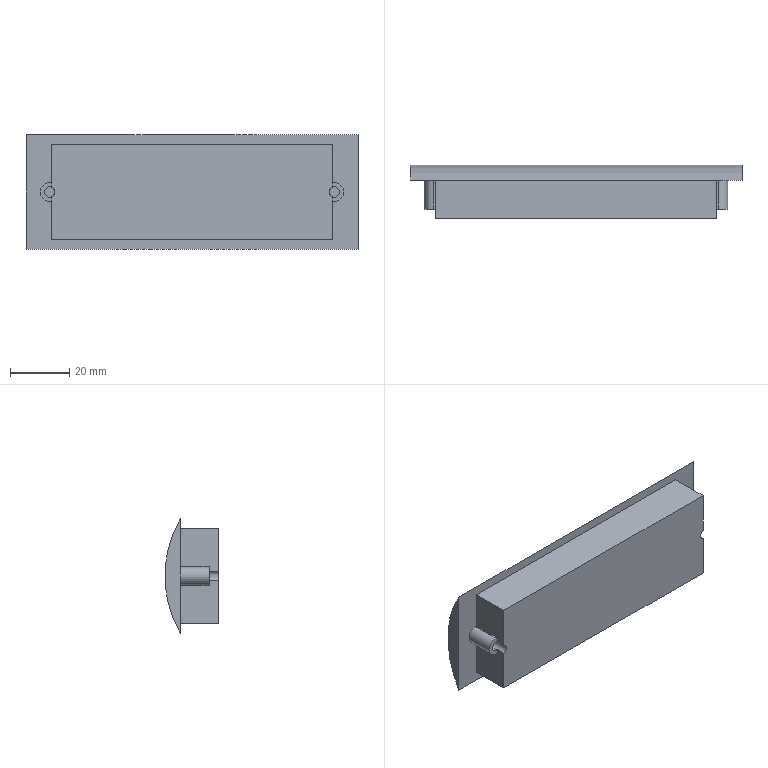Part | STEP file | LE-LLS-96B_LE0314013317 | 1 solid | 25 faces | box 112 x 18.2 x 38.5 mm | volume 54842 mm3 | plane 14 | cylinder 11 | commonest cylinder face diameters 6.3 x6 3.5 x4 76.462 x1
STEP:
#1=CARTESIAN_POINT('',(48.,-9.75,3.15));
#2=VERTEX_POINT('',#1);
#3=CARTESIAN_POINT('',(48.,-9.75,-3.15));
#4=VERTEX_POINT('',#3);
#5=CARTESIAN_POINT('',(48.,-9.75,0.));
#6=DIRECTION('',(0.,1.,0.));
#7=DIRECTION('',(0.,0.,1.));
#8=AXIS2_PLACEMENT_3D('',#5,#6,#7);
#9=CIRCLE('',#8,3.15);
#10=EDGE_CURVE('',#2,#4,#9,.T.);
#11=ORIENTED_EDGE('',*,*,#10,.T.);
#12=CARTESIAN_POINT('',(48.,0.,-3.15));
#13=VERTEX_POINT('',#12);
#14=CARTESIAN_POINT('',(48.,-9.75,-3.15));
#15=DIRECTION('',(0.,1.,0.));
#16=VECTOR('',#15,1000.);
#17=LINE('',#14,#16);
#18=EDGE_CURVE('',#4,#13,#17,.T.);
#19=ORIENTED_EDGE('',*,*,#18,.T.);
#20=CARTESIAN_POINT('',(48.,0.,3.15));
#21=VERTEX_POINT('',#20);
#22=CARTESIAN_POINT('',(48.,0.,0.));
#23=DIRECTION('',(0.,1.,0.));
#24=DIRECTION('',(0.,0.,1.));
#25=AXIS2_PLACEMENT_3D('',#22,#23,#24);
#26=CIRCLE('',#25,3.15);
#27=EDGE_CURVE('',#21,#13,#26,.T.);
#28=ORIENTED_EDGE('',*,*,#27,.F.);
#29=CARTESIAN_POINT('',(48.,-9.75,3.15));
#30=DIRECTION('',(0.,1.,0.));
#31=VECTOR('',#30,1000.);
#32=LINE('',#29,#31);
#33=EDGE_CURVE('',#2,#21,#32,.T.);
#34=ORIENTED_EDGE('',*,*,#33,.F.);
#35=EDGE_LOOP('',(#11,#19,#28,#34));
#36=FACE_OUTER_BOUND('',#35,.T.);
#37=CARTESIAN_POINT('',(48.,-9.75,0.));
#38=DIRECTION('',(0.,1.,0.));
#39=DIRECTION('',(0.,0.,1.));
#40=AXIS2_PLACEMENT_3D('',#37,#38,#39);
#41=CYLINDRICAL_SURFACE('',#40,3.15);
#42=ADVANCED_FACE('',(#36),#41,.T.);
#43=CARTESIAN_POINT('',(47.5,-9.75,3.11));
#44=VERTEX_POINT('',#43);
#45=CARTESIAN_POINT('',(48.,-9.75,0.));
#46=DIRECTION('',(0.,1.,0.));
#47=DIRECTION('',(0.,0.,1.));
#48=AXIS2_PLACEMENT_3D('',#45,#46,#47);
#49=CIRCLE('',#48,3.15);
#50=EDGE_CURVE('',#44,#2,#49,.T.);
#51=ORIENTED_EDGE('',*,*,#50,.T.);
#52=ORIENTED_EDGE('',*,*,#33,.T.);
#53=CARTESIAN_POINT('',(47.5,0.,3.11));
#54=VERTEX_POINT('',#53);
#55=CARTESIAN_POINT('',(48.,0.,0.));
#56=DIRECTION('',(0.,1.,0.));
#57=DIRECTION('',(0.,0.,1.));
#58=AXIS2_PLACEMENT_3D('',#55,#56,#57);
#59=CIRCLE('',#58,3.15);
#60=EDGE_CURVE('',#54,#21,#59,.T.);
#61=ORIENTED_EDGE('',*,*,#60,.F.);
#62=CARTESIAN_POINT('',(47.5,-13.,3.11));
#63=DIRECTION('',(0.,-1.,0.));
#64=VECTOR('',#63,1000.);
#65=LINE('',#62,#64);
#66=EDGE_CURVE('',#54,#44,#65,.T.);
#67=ORIENTED_EDGE('',*,*,#66,.T.);
#68=EDGE_LOOP('',(#51,#52,#61,#67));
#69=FACE_OUTER_BOUND('',#68,.T.);
#70=CARTESIAN_POINT('',(48.,-9.75,0.));
#71=DIRECTION('',(0.,1.,0.));
#72=DIRECTION('',(0.,0.,1.));
#73=AXIS2_PLACEMENT_3D('',#70,#71,#72);
#74=CYLINDRICAL_SURFACE('',#73,3.15);
#75=ADVANCED_FACE('',(#69),#74,.T.);
#76=CARTESIAN_POINT('',(-47.5,-9.75,-3.11));
#77=VERTEX_POINT('',#76);
#78=CARTESIAN_POINT('',(-48.,-9.75,-3.15));
#79=VERTEX_POINT('',#78);
#80=CARTESIAN_POINT('',(-48.,-9.75,0.));
#81=DIRECTION('',(0.,1.,0.));
#82=DIRECTION('',(0.,0.,1.));
#83=AXIS2_PLACEMENT_3D('',#80,#81,#82);
#84=CIRCLE('',#83,3.15);
#85=EDGE_CURVE('',#77,#79,#84,.T.);
#86=ORIENTED_EDGE('',*,*,#85,.T.);
#87=CARTESIAN_POINT('',(-48.,0.,-3.15));
#88=VERTEX_POINT('',#87);
#89=CARTESIAN_POINT('',(-48.,-9.75,-3.15));
#90=DIRECTION('',(0.,1.,0.));
#91=VECTOR('',#90,1000.);
#92=LINE('',#89,#91);
#93=EDGE_CURVE('',#79,#88,#92,.T.);
#94=ORIENTED_EDGE('',*,*,#93,.T.);
#95=CARTESIAN_POINT('',(-47.5,0.,-3.11));
#96=VERTEX_POINT('',#95);
#97=CARTESIAN_POINT('',(-48.,0.,0.));
#98=DIRECTION('',(0.,1.,0.));
#99=DIRECTION('',(0.,0.,1.));
#100=AXIS2_PLACEMENT_3D('',#97,#98,#99);
#101=CIRCLE('',#100,3.15);
#102=EDGE_CURVE('',#96,#88,#101,.T.);
#103=ORIENTED_EDGE('',*,*,#102,.F.);
#104=CARTESIAN_POINT('',(-47.5,-13.,-3.11));
#105=DIRECTION('',(0.,-1.,0.));
#106=VECTOR('',#105,1000.);
#107=LINE('',#104,#106);
#108=EDGE_CURVE('',#96,#77,#107,.T.);
#109=ORIENTED_EDGE('',*,*,#108,.T.);
#110=EDGE_LOOP('',(#86,#94,#103,#109));
#111=FACE_OUTER_BOUND('',#110,.T.);
#112=CARTESIAN_POINT('',(-48.,-9.75,0.));
#113=DIRECTION('',(0.,1.,0.));
#114=DIRECTION('',(0.,0.,1.));
#115=AXIS2_PLACEMENT_3D('',#112,#113,#114);
#116=CYLINDRICAL_SURFACE('',#115,3.15);
#117=ADVANCED_FACE('',(#111),#116,.T.);
#118=ORIENTED_EDGE('',*,*,#93,.F.);
#119=CARTESIAN_POINT('',(-48.,-9.75,3.15));
#120=VERTEX_POINT('',#119);
#121=CARTESIAN_POINT('',(-48.,-9.75,0.));
#122=DIRECTION('',(0.,1.,0.));
#123=DIRECTION('',(0.,0.,1.));
#124=AXIS2_PLACEMENT_3D('',#121,#122,#123);
#125=CIRCLE('',#124,3.15);
#126=EDGE_CURVE('',#79,#120,#125,.T.);
#127=ORIENTED_EDGE('',*,*,#126,.T.);
#128=CARTESIAN_POINT('',(-48.,0.,3.15));
#129=VERTEX_POINT('',#128);
#130=CARTESIAN_POINT('',(-48.,-9.75,3.15));
#131=DIRECTION('',(0.,1.,0.));
#132=VECTOR('',#131,1000.);
#133=LINE('',#130,#132);
#134=EDGE_CURVE('',#120,#129,#133,.T.);
#135=ORIENTED_EDGE('',*,*,#134,.T.);
#136=CARTESIAN_POINT('',(-48.,0.,0.));
#137=DIRECTION('',(0.,1.,0.));
#138=DIRECTION('',(0.,0.,1.));
#139=AXIS2_PLACEMENT_3D('',#136,#137,#138);
#140=CIRCLE('',#139,3.15);
#141=EDGE_CURVE('',#88,#129,#140,.T.);
#142=ORIENTED_EDGE('',*,*,#141,.F.);
#143=EDGE_LOOP('',(#118,#127,#135,#142));
#144=FACE_OUTER_BOUND('',#143,.T.);
#145=CARTESIAN_POINT('',(-48.,-9.75,0.));
#146=DIRECTION('',(0.,1.,0.));
#147=DIRECTION('',(0.,0.,1.));
#148=AXIS2_PLACEMENT_3D('',#145,#146,#147);
#149=CYLINDRICAL_SURFACE('',#148,3.15);
#150=ADVANCED_FACE('',(#144),#149,.T.);
#151=CARTESIAN_POINT('',(48.,0.,1.75));
#152=VERTEX_POINT('',#151);
#153=CARTESIAN_POINT('',(48.,0.,-1.75));
#154=VERTEX_POINT('',#153);
#155=CARTESIAN_POINT('',(48.,0.,0.));
#156=DIRECTION('',(0.,-1.,0.));
#157=DIRECTION('',(0.,0.,-1.));
#158=AXIS2_PLACEMENT_3D('',#155,#156,#157);
#159=CIRCLE('',#158,1.75);
#160=EDGE_CURVE('',#152,#154,#159,.T.);
#161=ORIENTED_EDGE('',*,*,#160,.F.);
#162=CARTESIAN_POINT('',(48.,-9.75,1.75));
#163=VERTEX_POINT('',#162);
#164=CARTESIAN_POINT('',(48.,0.,1.75));
#165=DIRECTION('',(0.,-1.,0.));
#166=VECTOR('',#165,1000.);
#167=LINE('',#164,#166);
#168=EDGE_CURVE('',#152,#163,#167,.T.);
#169=ORIENTED_EDGE('',*,*,#168,.T.);
#170=CARTESIAN_POINT('',(47.5,-9.75,1.677));
#171=VERTEX_POINT('',#170);
#172=CARTESIAN_POINT('',(48.,-9.75,0.));
#173=DIRECTION('',(0.,1.,0.));
#174=DIRECTION('',(0.,0.,-1.));
#175=AXIS2_PLACEMENT_3D('',#172,#173,#174);
#176=CIRCLE('',#175,1.75);
#177=EDGE_CURVE('',#171,#163,#176,.T.);
#178=ORIENTED_EDGE('',*,*,#177,.F.);
#179=CARTESIAN_POINT('',(47.5,-13.,1.677));
#180=VERTEX_POINT('',#179);
#181=CARTESIAN_POINT('',(47.5,-13.,1.677));
#182=DIRECTION('',(0.,-1.,0.));
#183=VECTOR('',#182,1000.);
#184=LINE('',#181,#183);
#185=EDGE_CURVE('',#171,#180,#184,.T.);
#186=ORIENTED_EDGE('',*,*,#185,.T.);
#187=CARTESIAN_POINT('',(47.5,-13.,-1.677));
#188=VERTEX_POINT('',#187);
#189=CARTESIAN_POINT('',(48.,-13.,0.));
#190=DIRECTION('',(0.,1.,0.));
#191=DIRECTION('',(0.,0.,-1.));
#192=AXIS2_PLACEMENT_3D('',#189,#190,#191);
#193=CIRCLE('',#192,1.75);
#194=EDGE_CURVE('',#188,#180,#193,.T.);
#195=ORIENTED_EDGE('',*,*,#194,.F.);
#196=CARTESIAN_POINT('',(47.5,-9.75,-1.677));
#197=VERTEX_POINT('',#196);
#198=CARTESIAN_POINT('',(47.5,-13.,-1.677));
#199=DIRECTION('',(0.,1.,0.));
#200=VECTOR('',#199,1000.);
#201=LINE('',#198,#200);
#202=EDGE_CURVE('',#188,#197,#201,.T.);
#203=ORIENTED_EDGE('',*,*,#202,.T.);
#204=CARTESIAN_POINT('',(48.,-9.75,-1.75));
#205=VERTEX_POINT('',#204);
#206=CARTESIAN_POINT('',(48.,-9.75,0.));
#207=DIRECTION('',(0.,1.,0.));
#208=DIRECTION('',(0.,0.,-1.));
#209=AXIS2_PLACEMENT_3D('',#206,#207,#208);
#210=CIRCLE('',#209,1.75);
#211=EDGE_CURVE('',#205,#197,#210,.T.);
#212=ORIENTED_EDGE('',*,*,#211,.F.);
#213=CARTESIAN_POINT('',(48.,0.,-1.75));
#214=DIRECTION('',(0.,-1.,0.));
#215=VECTOR('',#214,1000.);
#216=LINE('',#213,#215);
#217=EDGE_CURVE('',#154,#205,#216,.T.);
#218=ORIENTED_EDGE('',*,*,#217,.F.);
#219=EDGE_LOOP('',(#161,#169,#178,#186,#195,#203,#212,#218));
#220=FACE_OUTER_BOUND('',#219,.T.);
#221=CARTESIAN_POINT('',(48.,0.,0.));
#222=DIRECTION('',(0.,-1.,0.));
#223=DIRECTION('',(0.,0.,-1.));
#224=AXIS2_PLACEMENT_3D('',#221,#222,#223);
#225=CYLINDRICAL_SURFACE('',#224,1.75);
#226=ADVANCED_FACE('',(#220),#225,.F.);
#227=CARTESIAN_POINT('',(-48.,0.,1.75));
#228=VERTEX_POINT('',#227);
#229=CARTESIAN_POINT('',(-48.,0.,-1.75));
#230=VERTEX_POINT('',#229);
#231=CARTESIAN_POINT('',(-48.,0.,0.));
#232=DIRECTION('',(0.,-1.,0.));
#233=DIRECTION('',(0.,0.,-1.));
#234=AXIS2_PLACEMENT_3D('',#231,#232,#233);
#235=CIRCLE('',#234,1.75);
#236=EDGE_CURVE('',#228,#230,#235,.T.);
#237=ORIENTED_EDGE('',*,*,#236,.F.);
#238=CARTESIAN_POINT('',(-48.,-9.75,1.75));
#239=VERTEX_POINT('',#238);
#240=CARTESIAN_POINT('',(-48.,0.,1.75));
#241=DIRECTION('',(0.,-1.,0.));
#242=VECTOR('',#241,1000.);
#243=LINE('',#240,#242);
#244=EDGE_CURVE('',#228,#239,#243,.T.);
#245=ORIENTED_EDGE('',*,*,#244,.T.);
#246=CARTESIAN_POINT('',(-48.,-9.75,-1.75));
#247=VERTEX_POINT('',#246);
#248=CARTESIAN_POINT('',(-48.,-9.75,0.));
#249=DIRECTION('',(0.,1.,0.));
#250=DIRECTION('',(0.,0.,-1.));
#251=AXIS2_PLACEMENT_3D('',#248,#249,#250);
#252=CIRCLE('',#251,1.75);
#253=EDGE_CURVE('',#247,#239,#252,.T.);
#254=ORIENTED_EDGE('',*,*,#253,.F.);
#255=CARTESIAN_POINT('',(-48.,0.,-1.75));
#256=DIRECTION('',(0.,-1.,0.));
#257=VECTOR('',#256,1000.);
#258=LINE('',#255,#257);
#259=EDGE_CURVE('',#230,#247,#258,.T.);
#260=ORIENTED_EDGE('',*,*,#259,.F.);
#261=EDGE_LOOP('',(#237,#245,#254,#260));
#262=FACE_OUTER_BOUND('',#261,.T.);
#263=CARTESIAN_POINT('',(-48.,0.,0.));
#264=DIRECTION('',(0.,-1.,0.));
#265=DIRECTION('',(0.,0.,-1.));
#266=AXIS2_PLACEMENT_3D('',#263,#264,#265);
#267=CYLINDRICAL_SURFACE('',#266,1.75);
#268=ADVANCED_FACE('',(#262),#267,.F.);
#269=CARTESIAN_POINT('',(56.,0.,-19.25));
#270=VERTEX_POINT('',#269);
#271=CARTESIAN_POINT('',(-56.,0.,-19.25));
#272=VERTEX_POINT('',#271);
#273=CARTESIAN_POINT('',(56.,0.,-19.25));
#274=DIRECTION('',(-1.,0.,0.));
#275=VECTOR('',#274,1000.);
#276=LINE('',#273,#275);
#277=EDGE_CURVE('',#270,#272,#276,.T.);
#278=ORIENTED_EDGE('',*,*,#277,.T.);
#279=CARTESIAN_POINT('',(-56.,0.,19.25));
#280=VERTEX_POINT('',#279);
#281=CARTESIAN_POINT('',(-56.,-33.031,0.));
#282=DIRECTION('',(1.,0.,0.));
#283=DIRECTION('',(0.,-1.,0.));
#284=AXIS2_PLACEMENT_3D('',#281,#282,#283);
#285=CIRCLE('',#284,38.231);
#286=EDGE_CURVE('',#272,#280,#285,.T.);
#287=ORIENTED_EDGE('',*,*,#286,.T.);
#288=CARTESIAN_POINT('',(56.,0.,19.25));
#289=VERTEX_POINT('',#288);
#290=CARTESIAN_POINT('',(56.,0.,19.25));
#291=DIRECTION('',(1.,0.,0.));
#292=VECTOR('',#291,1000.);
#293=LINE('',#290,#292);
#294=EDGE_CURVE('',#280,#289,#293,.T.);
#295=ORIENTED_EDGE('',*,*,#294,.T.);
#296=CARTESIAN_POINT('',(56.,-33.031,0.));
#297=DIRECTION('',(-1.,0.,0.));
#298=DIRECTION('',(0.,-1.,0.));
#299=AXIS2_PLACEMENT_3D('',#296,#297,#298);
#300=CIRCLE('',#299,38.231);
#301=EDGE_CURVE('',#289,#270,#300,.T.);
#302=ORIENTED_EDGE('',*,*,#301,.T.);
#303=EDGE_LOOP('',(#278,#287,#295,#302));
#304=FACE_OUTER_BOUND('',#303,.T.);
#305=CARTESIAN_POINT('',(56.,-33.031,0.));
#306=DIRECTION('',(-1.,0.,0.));
#307=DIRECTION('',(0.,-1.,0.));
#308=AXIS2_PLACEMENT_3D('',#305,#306,#307);
#309=CYLINDRICAL_SURFACE('',#308,38.231);
#310=ADVANCED_FACE('',(#304),#309,.T.);
#311=ORIENTED_EDGE('',*,*,#286,.F.);
#312=CARTESIAN_POINT('',(-56.,0.,0.));
#313=DIRECTION('',(0.,0.,1.));
#314=VECTOR('',#313,1000.);
#315=LINE('',#312,#314);
#316=EDGE_CURVE('',#272,#280,#315,.T.);
#317=ORIENTED_EDGE('',*,*,#316,.T.);
#318=EDGE_LOOP('',(#311,#317));
#319=FACE_OUTER_BOUND('',#318,.T.);
#320=CARTESIAN_POINT('',(-56.,-33.031,0.));
#321=DIRECTION('',(-1.,0.,0.));
#322=DIRECTION('',(0.,0.,1.));
#323=AXIS2_PLACEMENT_3D('',#320,#321,#322);
#324=PLANE('',#323);
#325=ADVANCED_FACE('',(#319),#324,.T.);
#326=ORIENTED_EDGE('',*,*,#60,.T.);
#327=ORIENTED_EDGE('',*,*,#27,.T.);
#328=CARTESIAN_POINT('',(47.5,0.,-3.11));
#329=VERTEX_POINT('',#328);
#330=CARTESIAN_POINT('',(48.,0.,0.));
#331=DIRECTION('',(0.,1.,0.));
#332=DIRECTION('',(0.,0.,1.));
#333=AXIS2_PLACEMENT_3D('',#330,#331,#332);
#334=CIRCLE('',#333,3.15);
#335=EDGE_CURVE('',#13,#329,#334,.T.);
#336=ORIENTED_EDGE('',*,*,#335,.T.);
#337=CARTESIAN_POINT('',(47.5,0.,-16.));
#338=VERTEX_POINT('',#337);
#339=CARTESIAN_POINT('',(47.5,0.,-19.25));
#340=DIRECTION('',(0.,0.,-1.));
#341=VECTOR('',#340,1000.);
#342=LINE('',#339,#341);
#343=EDGE_CURVE('',#329,#338,#342,.T.);
#344=ORIENTED_EDGE('',*,*,#343,.T.);
#345=CARTESIAN_POINT('',(-47.5,0.,-16.));
#346=VERTEX_POINT('',#345);
#347=CARTESIAN_POINT('',(56.,0.,-16.));
#348=DIRECTION('',(-1.,0.,0.));
#349=VECTOR('',#348,1000.);
#350=LINE('',#347,#349);
#351=EDGE_CURVE('',#338,#346,#350,.T.);
#352=ORIENTED_EDGE('',*,*,#351,.T.);
#353=CARTESIAN_POINT('',(-47.5,0.,-19.25));
#354=DIRECTION('',(0.,0.,1.));
#355=VECTOR('',#354,1000.);
#356=LINE('',#353,#355);
#357=EDGE_CURVE('',#346,#96,#356,.T.);
#358=ORIENTED_EDGE('',*,*,#357,.T.);
#359=ORIENTED_EDGE('',*,*,#102,.T.);
#360=ORIENTED_EDGE('',*,*,#141,.T.);
#361=CARTESIAN_POINT('',(-47.5,0.,3.11));
#362=VERTEX_POINT('',#361);
#363=CARTESIAN_POINT('',(-48.,0.,0.));
#364=DIRECTION('',(0.,1.,0.));
#365=DIRECTION('',(0.,0.,1.));
#366=AXIS2_PLACEMENT_3D('',#363,#364,#365);
#367=CIRCLE('',#366,3.15);
#368=EDGE_CURVE('',#129,#362,#367,.T.);
#369=ORIENTED_EDGE('',*,*,#368,.T.);
#370=CARTESIAN_POINT('',(-47.5,0.,16.));
#371=VERTEX_POINT('',#370);
#372=CARTESIAN_POINT('',(-47.5,0.,-19.25));
#373=DIRECTION('',(0.,0.,1.));
#374=VECTOR('',#373,1000.);
#375=LINE('',#372,#374);
#376=EDGE_CURVE('',#362,#371,#375,.T.);
#377=ORIENTED_EDGE('',*,*,#376,.T.);
#378=CARTESIAN_POINT('',(47.5,0.,16.));
#379=VERTEX_POINT('',#378);
#380=CARTESIAN_POINT('',(56.,0.,16.));
#381=DIRECTION('',(1.,0.,0.));
#382=VECTOR('',#381,1000.);
#383=LINE('',#380,#382);
#384=EDGE_CURVE('',#371,#379,#383,.T.);
#385=ORIENTED_EDGE('',*,*,#384,.T.);
#386=CARTESIAN_POINT('',(47.5,0.,-19.25));
#387=DIRECTION('',(0.,0.,-1.));
#388=VECTOR('',#387,1000.);
#389=LINE('',#386,#388);
#390=EDGE_CURVE('',#379,#54,#389,.T.);
#391=ORIENTED_EDGE('',*,*,#390,.T.);
#392=EDGE_LOOP('',(#326,#327,#336,#344,#352,#358,#359,#360,#369,#377,#385,#391));
#393=FACE_BOUND('',#392,.T.);
#394=ORIENTED_EDGE('',*,*,#294,.F.);
#395=ORIENTED_EDGE('',*,*,#316,.F.);
#396=ORIENTED_EDGE('',*,*,#277,.F.);
#397=CARTESIAN_POINT('',(56.,0.,-19.25));
#398=DIRECTION('',(0.,0.,1.));
#399=VECTOR('',#398,1000.);
#400=LINE('',#397,#399);
#401=EDGE_CURVE('',#270,#289,#400,.T.);
#402=ORIENTED_EDGE('',*,*,#401,.T.);
#403=EDGE_LOOP('',(#394,#395,#396,#402));
#404=FACE_OUTER_BOUND('',#403,.T.);
#405=CARTESIAN_POINT('',(56.,0.,-19.25));
#406=DIRECTION('',(0.,-1.,0.));
#407=DIRECTION('',(1.,0.,0.));
#408=AXIS2_PLACEMENT_3D('',#405,#406,#407);
#409=PLANE('',#408);
#410=ADVANCED_FACE('',(#393,#404),#409,.T.);
#411=ORIENTED_EDGE('',*,*,#301,.F.);
#412=ORIENTED_EDGE('',*,*,#401,.F.);
#413=EDGE_LOOP('',(#411,#412));
#414=FACE_OUTER_BOUND('',#413,.T.);
#415=CARTESIAN_POINT('',(56.,-33.031,0.));
#416=DIRECTION('',(-1.,0.,0.));
#417=DIRECTION('',(0.,0.,1.));
#418=AXIS2_PLACEMENT_3D('',#415,#416,#417);
#419=PLANE('',#418);
#420=ADVANCED_FACE('',(#414),#419,.F.);
#421=CARTESIAN_POINT('',(47.5,-13.,-16.));
#422=VERTEX_POINT('',#421);
#423=CARTESIAN_POINT('',(47.5,-13.,-16.));
#424=DIRECTION('',(0.,0.,1.));
#425=VECTOR('',#424,1000.);
#426=LINE('',#423,#425);
#427=EDGE_CURVE('',#422,#188,#426,.T.);
#428=ORIENTED_EDGE('',*,*,#427,.F.);
#429=CARTESIAN_POINT('',(47.5,-13.,-16.));
#430=DIRECTION('',(0.,-1.,0.));
#431=VECTOR('',#430,1000.);
#432=LINE('',#429,#431);
#433=EDGE_CURVE('',#338,#422,#432,.T.);
#434=ORIENTED_EDGE('',*,*,#433,.F.);
#435=ORIENTED_EDGE('',*,*,#343,.F.);
#436=CARTESIAN_POINT('',(47.5,-9.75,-3.11));
#437=VERTEX_POINT('',#436);
#438=CARTESIAN_POINT('',(47.5,-13.,-3.11));
#439=DIRECTION('',(0.,1.,0.));
#440=VECTOR('',#439,1000.);
#441=LINE('',#438,#440);
#442=EDGE_CURVE('',#437,#329,#441,.T.);
#443=ORIENTED_EDGE('',*,*,#442,.F.);
#444=CARTESIAN_POINT('',(47.5,-9.75,0.));
#445=DIRECTION('',(0.,0.,-1.));
#446=VECTOR('',#445,1000.);
#447=LINE('',#444,#446);
#448=EDGE_CURVE('',#197,#437,#447,.T.);
#449=ORIENTED_EDGE('',*,*,#448,.F.);
#450=ORIENTED_EDGE('',*,*,#202,.F.);
#451=EDGE_LOOP('',(#428,#434,#435,#443,#449,#450));
#452=FACE_OUTER_BOUND('',#451,.T.);
#453=CARTESIAN_POINT('',(47.5,-13.,-16.));
#454=DIRECTION('',(-1.,0.,0.));
#455=DIRECTION('',(0.,0.,1.));
#456=AXIS2_PLACEMENT_3D('',#453,#454,#455);
#457=PLANE('',#456);
#458=ADVANCED_FACE('',(#452),#457,.F.);
#459=ORIENTED_EDGE('',*,*,#18,.F.);
#460=CARTESIAN_POINT('',(48.,-9.75,0.));
#461=DIRECTION('',(0.,1.,0.));
#462=DIRECTION('',(0.,0.,1.));
#463=AXIS2_PLACEMENT_3D('',#460,#461,#462);
#464=CIRCLE('',#463,3.15);
#465=EDGE_CURVE('',#4,#437,#464,.T.);
#466=ORIENTED_EDGE('',*,*,#465,.T.);
#467=ORIENTED_EDGE('',*,*,#442,.T.);
#468=ORIENTED_EDGE('',*,*,#335,.F.);
#469=EDGE_LOOP('',(#459,#466,#467,#468));
#470=FACE_OUTER_BOUND('',#469,.T.);
#471=CARTESIAN_POINT('',(48.,-9.75,0.));
#472=DIRECTION('',(0.,1.,0.));
#473=DIRECTION('',(0.,0.,1.));
#474=AXIS2_PLACEMENT_3D('',#471,#472,#473);
#475=CYLINDRICAL_SURFACE('',#474,3.15);
#476=ADVANCED_FACE('',(#470),#475,.T.);
#477=CARTESIAN_POINT('',(47.5,-9.75,-16.));
#478=DIRECTION('',(0.,0.,-1.));
#479=VECTOR('',#478,1000.);
#480=LINE('',#477,#479);
#481=EDGE_CURVE('',#44,#171,#480,.T.);
#482=ORIENTED_EDGE('',*,*,#481,.F.);
#483=ORIENTED_EDGE('',*,*,#66,.F.);
#484=ORIENTED_EDGE('',*,*,#390,.F.);
#485=CARTESIAN_POINT('',(47.5,-13.,16.));
#486=VERTEX_POINT('',#485);
#487=CARTESIAN_POINT('',(47.5,-13.,16.));
#488=DIRECTION('',(0.,1.,0.));
#489=VECTOR('',#488,1000.);
#490=LINE('',#487,#489);
#491=EDGE_CURVE('',#486,#379,#490,.T.);
#492=ORIENTED_EDGE('',*,*,#491,.F.);
#493=CARTESIAN_POINT('',(47.5,-13.,-16.));
#494=DIRECTION('',(0.,0.,1.));
#495=VECTOR('',#494,1000.);
#496=LINE('',#493,#495);
#497=EDGE_CURVE('',#180,#486,#496,.T.);
#498=ORIENTED_EDGE('',*,*,#497,.F.);
#499=ORIENTED_EDGE('',*,*,#185,.F.);
#500=EDGE_LOOP('',(#482,#483,#484,#492,#498,#499));
#501=FACE_OUTER_BOUND('',#500,.T.);
#502=CARTESIAN_POINT('',(47.5,-13.,-16.));
#503=DIRECTION('',(-1.,0.,0.));
#504=DIRECTION('',(0.,0.,1.));
#505=AXIS2_PLACEMENT_3D('',#502,#503,#504);
#506=PLANE('',#505);
#507=ADVANCED_FACE('',(#501),#506,.F.);
#508=CARTESIAN_POINT('',(-47.5,-13.,16.));
#509=VERTEX_POINT('',#508);
#510=CARTESIAN_POINT('',(-47.5,-13.,16.));
#511=DIRECTION('',(-1.,0.,0.));
#512=VECTOR('',#511,1000.);
#513=LINE('',#510,#512);
#514=EDGE_CURVE('',#486,#509,#513,.T.);
#515=ORIENTED_EDGE('',*,*,#514,.F.);
#516=ORIENTED_EDGE('',*,*,#491,.T.);
#517=ORIENTED_EDGE('',*,*,#384,.F.);
#518=CARTESIAN_POINT('',(-47.5,-13.,16.));
#519=DIRECTION('',(0.,1.,0.));
#520=VECTOR('',#519,1000.);
#521=LINE('',#518,#520);
#522=EDGE_CURVE('',#509,#371,#521,.T.);
#523=ORIENTED_EDGE('',*,*,#522,.F.);
#524=EDGE_LOOP('',(#515,#516,#517,#523));
#525=FACE_OUTER_BOUND('',#524,.T.);
#526=CARTESIAN_POINT('',(-47.5,-13.,16.));
#527=DIRECTION('',(0.,0.,-1.));
#528=DIRECTION('',(-1.,0.,0.));
#529=AXIS2_PLACEMENT_3D('',#526,#527,#528);
#530=PLANE('',#529);
#531=ADVANCED_FACE('',(#525),#530,.F.);
#532=ORIENTED_EDGE('',*,*,#522,.T.);
#533=ORIENTED_EDGE('',*,*,#376,.F.);
#534=CARTESIAN_POINT('',(-47.5,-9.75,3.11));
#535=VERTEX_POINT('',#534);
#536=CARTESIAN_POINT('',(-47.5,-13.,3.11));
#537=DIRECTION('',(0.,1.,0.));
#538=VECTOR('',#537,1000.);
#539=LINE('',#536,#538);
#540=EDGE_CURVE('',#535,#362,#539,.T.);
#541=ORIENTED_EDGE('',*,*,#540,.F.);
#542=CARTESIAN_POINT('',(-47.5,-9.75,1.677));
#543=VERTEX_POINT('',#542);
#544=CARTESIAN_POINT('',(-47.5,-9.75,0.));
#545=DIRECTION('',(0.,0.,1.));
#546=VECTOR('',#545,1000.);
#547=LINE('',#544,#546);
#548=EDGE_CURVE('',#543,#535,#547,.T.);
#549=ORIENTED_EDGE('',*,*,#548,.F.);
#550=CARTESIAN_POINT('',(-47.5,-13.,1.677));
#551=VERTEX_POINT('',#550);
#552=CARTESIAN_POINT('',(-47.5,-13.,1.677));
#553=DIRECTION('',(0.,1.,0.));
#554=VECTOR('',#553,1000.);
#555=LINE('',#552,#554);
#556=EDGE_CURVE('',#551,#543,#555,.T.);
#557=ORIENTED_EDGE('',*,*,#556,.F.);
#558=CARTESIAN_POINT('',(-47.5,-13.,-16.));
#559=DIRECTION('',(0.,0.,-1.));
#560=VECTOR('',#559,1000.);
#561=LINE('',#558,#560);
#562=EDGE_CURVE('',#509,#551,#561,.T.);
#563=ORIENTED_EDGE('',*,*,#562,.F.);
#564=EDGE_LOOP('',(#532,#533,#541,#549,#557,#563));
#565=FACE_OUTER_BOUND('',#564,.T.);
#566=CARTESIAN_POINT('',(-47.5,-13.,-16.));
#567=DIRECTION('',(1.,0.,0.));
#568=DIRECTION('',(0.,0.,-1.));
#569=AXIS2_PLACEMENT_3D('',#566,#567,#568);
#570=PLANE('',#569);
#571=ADVANCED_FACE('',(#565),#570,.F.);
#572=ORIENTED_EDGE('',*,*,#134,.F.);
#573=CARTESIAN_POINT('',(-48.,-9.75,0.));
#574=DIRECTION('',(0.,1.,0.));
#575=DIRECTION('',(0.,0.,1.));
#576=AXIS2_PLACEMENT_3D('',#573,#574,#575);
#577=CIRCLE('',#576,3.15);
#578=EDGE_CURVE('',#120,#535,#577,.T.);
#579=ORIENTED_EDGE('',*,*,#578,.T.);
#580=ORIENTED_EDGE('',*,*,#540,.T.);
#581=ORIENTED_EDGE('',*,*,#368,.F.);
#582=EDGE_LOOP('',(#572,#579,#580,#581));
#583=FACE_OUTER_BOUND('',#582,.T.);
#584=CARTESIAN_POINT('',(-48.,-9.75,0.));
#585=DIRECTION('',(0.,1.,0.));
#586=DIRECTION('',(0.,0.,1.));
#587=AXIS2_PLACEMENT_3D('',#584,#585,#586);
#588=CYLINDRICAL_SURFACE('',#587,3.15);
#589=ADVANCED_FACE('',(#583),#588,.T.);
#590=ORIENTED_EDGE('',*,*,#108,.F.);
#591=ORIENTED_EDGE('',*,*,#357,.F.);
#592=CARTESIAN_POINT('',(-47.5,-13.,-16.));
#593=VERTEX_POINT('',#592);
#594=CARTESIAN_POINT('',(-47.5,-13.,-16.));
#595=DIRECTION('',(0.,1.,0.));
#596=VECTOR('',#595,1000.);
#597=LINE('',#594,#596);
#598=EDGE_CURVE('',#593,#346,#597,.T.);
#599=ORIENTED_EDGE('',*,*,#598,.F.);
#600=CARTESIAN_POINT('',(-47.5,-13.,-1.677));
#601=VERTEX_POINT('',#600);
#602=CARTESIAN_POINT('',(-47.5,-13.,-16.));
#603=DIRECTION('',(0.,0.,-1.));
#604=VECTOR('',#603,1000.);
#605=LINE('',#602,#604);
#606=EDGE_CURVE('',#601,#593,#605,.T.);
#607=ORIENTED_EDGE('',*,*,#606,.F.);
#608=CARTESIAN_POINT('',(-47.5,-9.75,-1.677));
#609=VERTEX_POINT('',#608);
#610=CARTESIAN_POINT('',(-47.5,-13.,-1.677));
#611=DIRECTION('',(0.,-1.,0.));
#612=VECTOR('',#611,1000.);
#613=LINE('',#610,#612);
#614=EDGE_CURVE('',#609,#601,#613,.T.);
#615=ORIENTED_EDGE('',*,*,#614,.F.);
#616=CARTESIAN_POINT('',(-47.5,-9.75,-16.));
#617=DIRECTION('',(0.,0.,1.));
#618=VECTOR('',#617,1000.);
#619=LINE('',#616,#618);
#620=EDGE_CURVE('',#77,#609,#619,.T.);
#621=ORIENTED_EDGE('',*,*,#620,.F.);
#622=EDGE_LOOP('',(#590,#591,#599,#607,#615,#621));
#623=FACE_OUTER_BOUND('',#622,.T.);
#624=CARTESIAN_POINT('',(-47.5,-13.,-16.));
#625=DIRECTION('',(1.,0.,0.));
#626=DIRECTION('',(0.,0.,-1.));
#627=AXIS2_PLACEMENT_3D('',#624,#625,#626);
#628=PLANE('',#627);
#629=ADVANCED_FACE('',(#623),#628,.F.);
#630=CARTESIAN_POINT('',(-47.5,-13.,-16.));
#631=DIRECTION('',(1.,0.,0.));
#632=VECTOR('',#631,1000.);
#633=LINE('',#630,#632);
#634=EDGE_CURVE('',#593,#422,#633,.T.);
#635=ORIENTED_EDGE('',*,*,#634,.F.);
#636=ORIENTED_EDGE('',*,*,#598,.T.);
#637=ORIENTED_EDGE('',*,*,#351,.F.);
#638=ORIENTED_EDGE('',*,*,#433,.T.);
#639=EDGE_LOOP('',(#635,#636,#637,#638));
#640=FACE_OUTER_BOUND('',#639,.T.);
#641=CARTESIAN_POINT('',(-47.5,-13.,-16.));
#642=DIRECTION('',(0.,0.,1.));
#643=DIRECTION('',(1.,0.,0.));
#644=AXIS2_PLACEMENT_3D('',#641,#642,#643);
#645=PLANE('',#644);
#646=ADVANCED_FACE('',(#640),#645,.F.);
#647=ORIENTED_EDGE('',*,*,#168,.F.);
#648=CARTESIAN_POINT('',(48.,0.,0.));
#649=DIRECTION('',(0.,-1.,0.));
#650=DIRECTION('',(0.,0.,-1.));
#651=AXIS2_PLACEMENT_3D('',#648,#649,#650);
#652=CIRCLE('',#651,1.75);
#653=EDGE_CURVE('',#154,#152,#652,.T.);
#654=ORIENTED_EDGE('',*,*,#653,.F.);
#655=ORIENTED_EDGE('',*,*,#217,.T.);
#656=CARTESIAN_POINT('',(48.,-9.75,0.));
#657=DIRECTION('',(0.,1.,0.));
#658=DIRECTION('',(0.,0.,-1.));
#659=AXIS2_PLACEMENT_3D('',#656,#657,#658);
#660=CIRCLE('',#659,1.75);
#661=EDGE_CURVE('',#163,#205,#660,.T.);
#662=ORIENTED_EDGE('',*,*,#661,.F.);
#663=EDGE_LOOP('',(#647,#654,#655,#662));
#664=FACE_OUTER_BOUND('',#663,.T.);
#665=CARTESIAN_POINT('',(48.,0.,0.));
#666=DIRECTION('',(0.,-1.,0.));
#667=DIRECTION('',(0.,0.,-1.));
#668=AXIS2_PLACEMENT_3D('',#665,#666,#667);
#669=CYLINDRICAL_SURFACE('',#668,1.75);
#670=ADVANCED_FACE('',(#664),#669,.F.);
#671=ORIENTED_EDGE('',*,*,#427,.T.);
#672=ORIENTED_EDGE('',*,*,#194,.T.);
#673=ORIENTED_EDGE('',*,*,#497,.T.);
#674=ORIENTED_EDGE('',*,*,#514,.T.);
#675=ORIENTED_EDGE('',*,*,#562,.T.);
#676=CARTESIAN_POINT('',(-48.,-13.,0.));
#677=DIRECTION('',(0.,1.,0.));
#678=DIRECTION('',(0.,0.,-1.));
#679=AXIS2_PLACEMENT_3D('',#676,#677,#678);
#680=CIRCLE('',#679,1.75);
#681=EDGE_CURVE('',#551,#601,#680,.T.);
#682=ORIENTED_EDGE('',*,*,#681,.T.);
#683=ORIENTED_EDGE('',*,*,#606,.T.);
#684=ORIENTED_EDGE('',*,*,#634,.T.);
#685=EDGE_LOOP('',(#671,#672,#673,#674,#675,#682,#683,#684));
#686=FACE_OUTER_BOUND('',#685,.T.);
#687=CARTESIAN_POINT('',(47.5,-13.,-16.));
#688=DIRECTION('',(0.,-1.,0.));
#689=DIRECTION('',(0.,0.,-1.));
#690=AXIS2_PLACEMENT_3D('',#687,#688,#689);
#691=PLANE('',#690);
#692=ADVANCED_FACE('',(#686),#691,.T.);
#693=ORIENTED_EDGE('',*,*,#50,.F.);
#694=ORIENTED_EDGE('',*,*,#481,.T.);
#695=ORIENTED_EDGE('',*,*,#177,.T.);
#696=ORIENTED_EDGE('',*,*,#661,.T.);
#697=ORIENTED_EDGE('',*,*,#211,.T.);
#698=ORIENTED_EDGE('',*,*,#448,.T.);
#699=ORIENTED_EDGE('',*,*,#465,.F.);
#700=ORIENTED_EDGE('',*,*,#10,.F.);
#701=EDGE_LOOP('',(#693,#694,#695,#696,#697,#698,#699,#700));
#702=FACE_OUTER_BOUND('',#701,.T.);
#703=CARTESIAN_POINT('',(48.,-9.75,0.));
#704=DIRECTION('',(0.,-1.,0.));
#705=DIRECTION('',(1.,0.,0.));
#706=AXIS2_PLACEMENT_3D('',#703,#704,#705);
#707=PLANE('',#706);
#708=ADVANCED_FACE('',(#702),#707,.T.);
#709=ORIENTED_EDGE('',*,*,#244,.F.);
#710=CARTESIAN_POINT('',(-48.,0.,0.));
#711=DIRECTION('',(0.,-1.,0.));
#712=DIRECTION('',(0.,0.,-1.));
#713=AXIS2_PLACEMENT_3D('',#710,#711,#712);
#714=CIRCLE('',#713,1.75);
#715=EDGE_CURVE('',#230,#228,#714,.T.);
#716=ORIENTED_EDGE('',*,*,#715,.F.);
#717=ORIENTED_EDGE('',*,*,#259,.T.);
#718=CARTESIAN_POINT('',(-48.,-9.75,0.));
#719=DIRECTION('',(0.,1.,0.));
#720=DIRECTION('',(0.,0.,-1.));
#721=AXIS2_PLACEMENT_3D('',#718,#719,#720);
#722=CIRCLE('',#721,1.75);
#723=EDGE_CURVE('',#609,#247,#722,.T.);
#724=ORIENTED_EDGE('',*,*,#723,.F.);
#725=ORIENTED_EDGE('',*,*,#614,.T.);
#726=ORIENTED_EDGE('',*,*,#681,.F.);
#727=ORIENTED_EDGE('',*,*,#556,.T.);
#728=CARTESIAN_POINT('',(-48.,-9.75,0.));
#729=DIRECTION('',(0.,1.,0.));
#730=DIRECTION('',(0.,0.,-1.));
#731=AXIS2_PLACEMENT_3D('',#728,#729,#730);
#732=CIRCLE('',#731,1.75);
#733=EDGE_CURVE('',#239,#543,#732,.T.);
#734=ORIENTED_EDGE('',*,*,#733,.F.);
#735=EDGE_LOOP('',(#709,#716,#717,#724,#725,#726,#727,#734));
#736=FACE_OUTER_BOUND('',#735,.T.);
#737=CARTESIAN_POINT('',(-48.,0.,0.));
#738=DIRECTION('',(0.,-1.,0.));
#739=DIRECTION('',(0.,0.,-1.));
#740=AXIS2_PLACEMENT_3D('',#737,#738,#739);
#741=CYLINDRICAL_SURFACE('',#740,1.75);
#742=ADVANCED_FACE('',(#736),#741,.F.);
#743=ORIENTED_EDGE('',*,*,#548,.T.);
#744=ORIENTED_EDGE('',*,*,#578,.F.);
#745=ORIENTED_EDGE('',*,*,#126,.F.);
#746=ORIENTED_EDGE('',*,*,#85,.F.);
#747=ORIENTED_EDGE('',*,*,#620,.T.);
#748=ORIENTED_EDGE('',*,*,#723,.T.);
#749=ORIENTED_EDGE('',*,*,#253,.T.);
#750=ORIENTED_EDGE('',*,*,#733,.T.);
#751=EDGE_LOOP('',(#743,#744,#745,#746,#747,#748,#749,#750));
#752=FACE_OUTER_BOUND('',#751,.T.);
#753=CARTESIAN_POINT('',(-48.,-9.75,0.));
#754=DIRECTION('',(0.,-1.,0.));
#755=DIRECTION('',(1.,0.,0.));
#756=AXIS2_PLACEMENT_3D('',#753,#754,#755);
#757=PLANE('',#756);
#758=ADVANCED_FACE('',(#752),#757,.T.);
#759=ORIENTED_EDGE('',*,*,#653,.T.);
#760=ORIENTED_EDGE('',*,*,#160,.T.);
#761=EDGE_LOOP('',(#759,#760));
#762=FACE_OUTER_BOUND('',#761,.T.);
#763=CARTESIAN_POINT('',(48.,0.,0.));
#764=DIRECTION('',(0.,-1.,0.));
#765=DIRECTION('',(1.,0.,0.));
#766=AXIS2_PLACEMENT_3D('',#763,#764,#765);
#767=PLANE('',#766);
#768=ADVANCED_FACE('',(#762),#767,.T.);
#769=ORIENTED_EDGE('',*,*,#715,.T.);
#770=ORIENTED_EDGE('',*,*,#236,.T.);
#771=EDGE_LOOP('',(#769,#770));
#772=FACE_OUTER_BOUND('',#771,.T.);
#773=CARTESIAN_POINT('',(-48.,0.,0.));
#774=DIRECTION('',(0.,-1.,0.));
#775=DIRECTION('',(1.,0.,0.));
#776=AXIS2_PLACEMENT_3D('',#773,#774,#775);
#777=PLANE('',#776);
#778=ADVANCED_FACE('',(#772),#777,.T.);
#779=CLOSED_SHELL('',(#42,#75,#117,#150,#226,#268,#310,#325,#410,#420,#458,#476,#507,#531,#571,#589,#629,#646,#670,#692,#708,#742,#758,#768,#778));
#780=MANIFOLD_SOLID_BREP('',#779);
#781=CARTESIAN_POINT('',(0.,0.,0.));
#782=DIRECTION('',(0.,0.,1.));
#783=DIRECTION('',(1.,0.,0.));
#784=AXIS2_PLACEMENT_3D('',#781,#782,#783);
#785=(LENGTH_UNIT()NAMED_UNIT(*)SI_UNIT(.MILLI.,.METRE.));
#786=UNCERTAINTY_MEASURE_WITH_UNIT(LENGTH_MEASURE(0.00001),#785,'','');
#787=(NAMED_UNIT(*)PLANE_ANGLE_UNIT()SI_UNIT($,.RADIAN.));
#788=(NAMED_UNIT(*)SI_UNIT($,.STERADIAN.)SOLID_ANGLE_UNIT());
#789=(GEOMETRIC_REPRESENTATION_CONTEXT(3)GLOBAL_UNCERTAINTY_ASSIGNED_CONTEXT((#786))GLOBAL_UNIT_ASSIGNED_CONTEXT((#785,#787,#788))REPRESENTATION_CONTEXT('',''));
#790=ADVANCED_BREP_SHAPE_REPRESENTATION('',(#780,#784),#789);